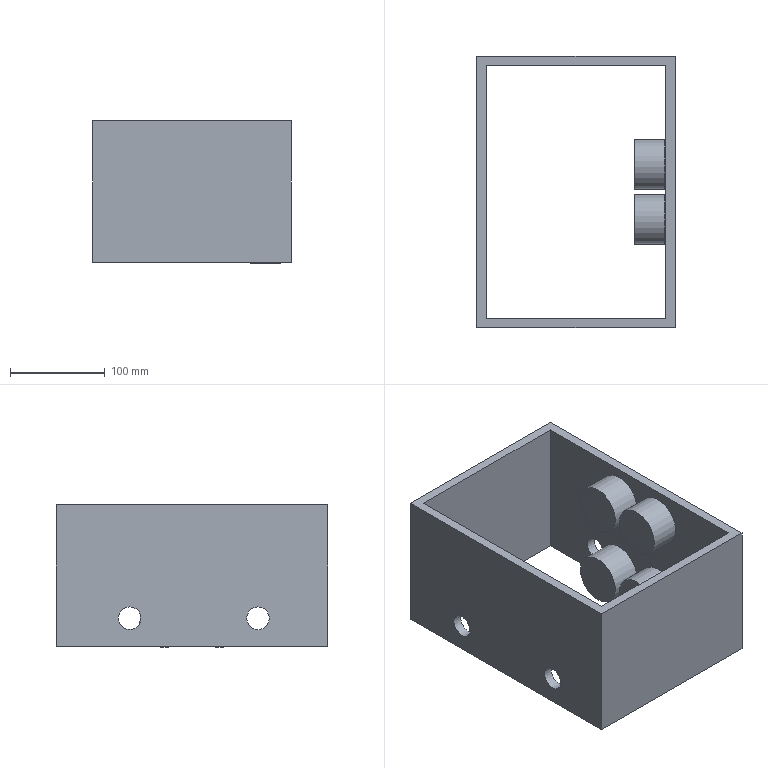Part | NX | features BREP 5 | 5 solids | 26 faces | box 209.8 x 286.897 x 151.129 mm | volume 1686526 mm3 | plane 18 | cylinder 8 | commonest cylinder face diameters 24 x4 52.257 x4
STEP:
#1=CARTESIAN_POINT('',(376.9,890.205,101.));
#2=VERTEX_POINT('',#1);
#3=CARTESIAN_POINT('',(376.9,864.077,101.));
#4=DIRECTION('',(1.,0.,0.));
#5=DIRECTION('',(0.,1.,0.));
#6=AXIS2_PLACEMENT_3D('',#3,#4,#5);
#7=CIRCLE('',#6,26.129);
#8=EDGE_CURVE('',#2,#2,#7,.T.);
#9=ORIENTED_EDGE('',*,*,#8,.T.);
#10=EDGE_LOOP('',(#9));
#11=FACE_BOUND('',#10,.T.);
#12=CARTESIAN_POINT('',(408.9,890.205,101.));
#13=VERTEX_POINT('',#12);
#14=CARTESIAN_POINT('',(408.9,864.077,101.));
#15=DIRECTION('',(1.,0.,0.));
#16=DIRECTION('',(0.,1.,0.));
#17=AXIS2_PLACEMENT_3D('',#14,#15,#16);
#18=CIRCLE('',#17,26.129);
#19=EDGE_CURVE('',#13,#13,#18,.T.);
#20=ORIENTED_EDGE('',*,*,#19,.F.);
#21=EDGE_LOOP('',(#20));
#22=FACE_BOUND('',#21,.T.);
#23=CARTESIAN_POINT('',(376.9,864.077,101.));
#24=DIRECTION('',(1.,0.,0.));
#25=DIRECTION('',(0.,0.,1.));
#26=AXIS2_PLACEMENT_3D('',#23,#24,#25);
#27=CYLINDRICAL_SURFACE('',#26,26.129);
#28=ADVANCED_FACE('',(#11,#22),#27,.T.);
#29=ORIENTED_EDGE('',*,*,#8,.F.);
#30=EDGE_LOOP('',(#29));
#31=FACE_BOUND('',#30,.T.);
#32=CARTESIAN_POINT('',(376.9,864.077,101.));
#33=DIRECTION('',(1.,0.,0.));
#34=DIRECTION('',(0.,0.,1.));
#35=AXIS2_PLACEMENT_3D('',#32,#33,#34);
#36=PLANE('',#35);
#37=ADVANCED_FACE('',(#31),#36,.F.);
#38=ORIENTED_EDGE('',*,*,#19,.T.);
#39=EDGE_LOOP('',(#38));
#40=FACE_BOUND('',#39,.T.);
#41=CARTESIAN_POINT('',(408.9,864.077,101.));
#42=DIRECTION('',(1.,0.,0.));
#43=DIRECTION('',(0.,0.,1.));
#44=AXIS2_PLACEMENT_3D('',#41,#42,#43);
#45=PLANE('',#44);
#46=ADVANCED_FACE('',(#40),#45,.T.);
#47=CLOSED_SHELL('',(#28,#37,#46));
#48=MANIFOLD_SOLID_BREP('',#47);
#49=CARTESIAN_POINT('',(210.1,691.509,136.));
#50=VERTEX_POINT('',#49);
#51=CARTESIAN_POINT('',(210.1,978.406,136.));
#52=VERTEX_POINT('',#51);
#53=CARTESIAN_POINT('',(210.1,943.406,136.));
#54=DIRECTION('',(0.,1.,0.));
#55=VECTOR('',#54,1000.);
#56=LINE('',#53,#55);
#57=EDGE_CURVE('',#50,#52,#56,.T.);
#58=ORIENTED_EDGE('',*,*,#57,.T.);
#59=CARTESIAN_POINT('',(210.1,978.406,-14.));
#60=VERTEX_POINT('',#59);
#61=CARTESIAN_POINT('',(210.1,978.406,-14.));
#62=DIRECTION('',(0.,0.,-1.));
#63=VECTOR('',#62,1000.);
#64=LINE('',#61,#63);
#65=EDGE_CURVE('',#52,#60,#64,.T.);
#66=ORIENTED_EDGE('',*,*,#65,.T.);
#67=CARTESIAN_POINT('',(210.1,691.509,-14.));
#68=VERTEX_POINT('',#67);
#69=CARTESIAN_POINT('',(210.1,943.406,-14.));
#70=DIRECTION('',(0.,-1.,0.));
#71=VECTOR('',#70,1000.);
#72=LINE('',#69,#71);
#73=EDGE_CURVE('',#60,#68,#72,.T.);
#74=ORIENTED_EDGE('',*,*,#73,.T.);
#75=CARTESIAN_POINT('',(210.1,691.509,-14.));
#76=DIRECTION('',(0.,0.,1.));
#77=VECTOR('',#76,1000.);
#78=LINE('',#75,#77);
#79=EDGE_CURVE('',#68,#50,#78,.T.);
#80=ORIENTED_EDGE('',*,*,#79,.T.);
#81=EDGE_LOOP('',(#58,#66,#74,#80));
#82=FACE_BOUND('',#81,.T.);
#83=CARTESIAN_POINT('',(210.1,765.15,27.85));
#84=VERTEX_POINT('',#83);
#85=CARTESIAN_POINT('',(210.1,765.15,15.85));
#86=DIRECTION('',(-1.,0.,0.));
#87=DIRECTION('',(0.,0.,1.));
#88=AXIS2_PLACEMENT_3D('',#85,#86,#87);
#89=CIRCLE('',#88,12.);
#90=EDGE_CURVE('',#84,#84,#89,.T.);
#91=ORIENTED_EDGE('',*,*,#90,.F.);
#92=EDGE_LOOP('',(#91));
#93=FACE_BOUND('',#92,.T.);
#94=CARTESIAN_POINT('',(210.1,900.853,27.85));
#95=VERTEX_POINT('',#94);
#96=CARTESIAN_POINT('',(210.1,900.853,15.85));
#97=DIRECTION('',(1.,0.,0.));
#98=DIRECTION('',(0.,0.,1.));
#99=AXIS2_PLACEMENT_3D('',#96,#97,#98);
#100=CIRCLE('',#99,12.);
#101=EDGE_CURVE('',#95,#95,#100,.T.);
#102=ORIENTED_EDGE('',*,*,#101,.T.);
#103=EDGE_LOOP('',(#102));
#104=FACE_BOUND('',#103,.T.);
#105=CARTESIAN_POINT('',(210.1,943.406,-14.));
#106=DIRECTION('',(-1.,0.,0.));
#107=DIRECTION('',(0.,0.,-1.));
#108=AXIS2_PLACEMENT_3D('',#105,#106,#107);
#109=PLANE('',#108);
#110=ADVANCED_FACE('',(#82,#93,#104),#109,.T.);
#111=CARTESIAN_POINT('',(419.9,978.406,136.));
#112=VERTEX_POINT('',#111);
#113=CARTESIAN_POINT('',(419.9,691.509,136.));
#114=VERTEX_POINT('',#113);
#115=CARTESIAN_POINT('',(419.9,726.509,136.));
#116=DIRECTION('',(0.,-1.,0.));
#117=VECTOR('',#116,1000.);
#118=LINE('',#115,#117);
#119=EDGE_CURVE('',#112,#114,#118,.T.);
#120=ORIENTED_EDGE('',*,*,#119,.T.);
#121=CARTESIAN_POINT('',(419.9,691.509,-14.));
#122=VERTEX_POINT('',#121);
#123=CARTESIAN_POINT('',(419.9,691.509,-14.));
#124=DIRECTION('',(0.,0.,1.));
#125=VECTOR('',#124,1000.);
#126=LINE('',#123,#125);
#127=EDGE_CURVE('',#122,#114,#126,.T.);
#128=ORIENTED_EDGE('',*,*,#127,.F.);
#129=CARTESIAN_POINT('',(419.9,978.406,-14.));
#130=VERTEX_POINT('',#129);
#131=CARTESIAN_POINT('',(419.9,923.406,-14.));
#132=DIRECTION('',(0.,1.,0.));
#133=VECTOR('',#132,1000.);
#134=LINE('',#131,#133);
#135=EDGE_CURVE('',#122,#130,#134,.T.);
#136=ORIENTED_EDGE('',*,*,#135,.T.);
#137=CARTESIAN_POINT('',(419.9,978.406,-14.));
#138=DIRECTION('',(0.,0.,1.));
#139=VECTOR('',#138,1000.);
#140=LINE('',#137,#139);
#141=EDGE_CURVE('',#130,#112,#140,.T.);
#142=ORIENTED_EDGE('',*,*,#141,.T.);
#143=EDGE_LOOP('',(#120,#128,#136,#142));
#144=FACE_BOUND('',#143,.T.);
#145=CARTESIAN_POINT('',(419.9,765.15,3.85));
#146=VERTEX_POINT('',#145);
#147=CARTESIAN_POINT('',(419.9,765.15,15.85));
#148=DIRECTION('',(1.,0.,0.));
#149=DIRECTION('',(0.,0.,-1.));
#150=AXIS2_PLACEMENT_3D('',#147,#148,#149);
#151=CIRCLE('',#150,12.);
#152=EDGE_CURVE('',#146,#146,#151,.T.);
#153=ORIENTED_EDGE('',*,*,#152,.F.);
#154=EDGE_LOOP('',(#153));
#155=FACE_BOUND('',#154,.T.);
#156=CARTESIAN_POINT('',(419.9,900.853,3.85));
#157=VERTEX_POINT('',#156);
#158=CARTESIAN_POINT('',(419.9,900.853,15.85));
#159=DIRECTION('',(-1.,0.,0.));
#160=DIRECTION('',(0.,0.,-1.));
#161=AXIS2_PLACEMENT_3D('',#158,#159,#160);
#162=CIRCLE('',#161,12.);
#163=EDGE_CURVE('',#157,#157,#162,.T.);
#164=ORIENTED_EDGE('',*,*,#163,.T.);
#165=EDGE_LOOP('',(#164));
#166=FACE_BOUND('',#165,.T.);
#167=CARTESIAN_POINT('',(419.9,726.509,-14.));
#168=DIRECTION('',(1.,0.,0.));
#169=DIRECTION('',(0.,0.,1.));
#170=AXIS2_PLACEMENT_3D('',#167,#168,#169);
#171=PLANE('',#170);
#172=ADVANCED_FACE('',(#144,#155,#166),#171,.T.);
#173=CARTESIAN_POINT('',(220.1,765.15,27.85));
#174=VERTEX_POINT('',#173);
#175=CARTESIAN_POINT('',(220.1,765.15,15.85));
#176=DIRECTION('',(-1.,0.,0.));
#177=DIRECTION('',(0.,0.,1.));
#178=AXIS2_PLACEMENT_3D('',#175,#176,#177);
#179=CIRCLE('',#178,12.);
#180=EDGE_CURVE('',#174,#174,#179,.T.);
#181=ORIENTED_EDGE('',*,*,#180,.T.);
#182=EDGE_LOOP('',(#181));
#183=FACE_BOUND('',#182,.T.);
#184=CARTESIAN_POINT('',(220.1,701.509,136.));
#185=VERTEX_POINT('',#184);
#186=CARTESIAN_POINT('',(220.1,968.406,136.));
#187=VERTEX_POINT('',#186);
#188=CARTESIAN_POINT('',(220.1,943.406,136.));
#189=DIRECTION('',(0.,1.,0.));
#190=VECTOR('',#189,1000.);
#191=LINE('',#188,#190);
#192=EDGE_CURVE('',#185,#187,#191,.T.);
#193=ORIENTED_EDGE('',*,*,#192,.F.);
#194=CARTESIAN_POINT('',(220.1,701.509,-14.));
#195=VERTEX_POINT('',#194);
#196=CARTESIAN_POINT('',(220.1,701.509,-14.));
#197=DIRECTION('',(0.,0.,1.));
#198=VECTOR('',#197,1000.);
#199=LINE('',#196,#198);
#200=EDGE_CURVE('',#195,#185,#199,.T.);
#201=ORIENTED_EDGE('',*,*,#200,.F.);
#202=CARTESIAN_POINT('',(220.1,968.406,-14.));
#203=VERTEX_POINT('',#202);
#204=CARTESIAN_POINT('',(220.1,943.406,-14.));
#205=DIRECTION('',(0.,-1.,0.));
#206=VECTOR('',#205,1000.);
#207=LINE('',#204,#206);
#208=EDGE_CURVE('',#203,#195,#207,.T.);
#209=ORIENTED_EDGE('',*,*,#208,.F.);
#210=CARTESIAN_POINT('',(220.1,968.406,-14.));
#211=DIRECTION('',(0.,0.,-1.));
#212=VECTOR('',#211,1000.);
#213=LINE('',#210,#212);
#214=EDGE_CURVE('',#187,#203,#213,.T.);
#215=ORIENTED_EDGE('',*,*,#214,.F.);
#216=EDGE_LOOP('',(#193,#201,#209,#215));
#217=FACE_BOUND('',#216,.T.);
#218=CARTESIAN_POINT('',(220.1,900.853,27.85));
#219=VERTEX_POINT('',#218);
#220=CARTESIAN_POINT('',(220.1,900.853,15.85));
#221=DIRECTION('',(1.,0.,0.));
#222=DIRECTION('',(0.,0.,1.));
#223=AXIS2_PLACEMENT_3D('',#220,#221,#222);
#224=CIRCLE('',#223,12.);
#225=EDGE_CURVE('',#219,#219,#224,.T.);
#226=ORIENTED_EDGE('',*,*,#225,.F.);
#227=EDGE_LOOP('',(#226));
#228=FACE_BOUND('',#227,.T.);
#229=CARTESIAN_POINT('',(220.1,943.406,-14.));
#230=DIRECTION('',(-1.,0.,0.));
#231=DIRECTION('',(0.,0.,-1.));
#232=AXIS2_PLACEMENT_3D('',#229,#230,#231);
#233=PLANE('',#232);
#234=ADVANCED_FACE('',(#183,#217,#228),#233,.F.);
#235=CARTESIAN_POINT('',(409.9,765.15,3.85));
#236=VERTEX_POINT('',#235);
#237=CARTESIAN_POINT('',(409.9,765.15,15.85));
#238=DIRECTION('',(1.,0.,0.));
#239=DIRECTION('',(0.,0.,-1.));
#240=AXIS2_PLACEMENT_3D('',#237,#238,#239);
#241=CIRCLE('',#240,12.);
#242=EDGE_CURVE('',#236,#236,#241,.T.);
#243=ORIENTED_EDGE('',*,*,#242,.T.);
#244=EDGE_LOOP('',(#243));
#245=FACE_BOUND('',#244,.T.);
#246=CARTESIAN_POINT('',(409.9,968.406,136.));
#247=VERTEX_POINT('',#246);
#248=CARTESIAN_POINT('',(409.9,701.509,136.));
#249=VERTEX_POINT('',#248);
#250=CARTESIAN_POINT('',(409.9,726.509,136.));
#251=DIRECTION('',(0.,-1.,0.));
#252=VECTOR('',#251,1000.);
#253=LINE('',#250,#252);
#254=EDGE_CURVE('',#247,#249,#253,.T.);
#255=ORIENTED_EDGE('',*,*,#254,.F.);
#256=CARTESIAN_POINT('',(409.9,968.406,-14.));
#257=VERTEX_POINT('',#256);
#258=CARTESIAN_POINT('',(409.9,968.406,-14.));
#259=DIRECTION('',(0.,0.,1.));
#260=VECTOR('',#259,1000.);
#261=LINE('',#258,#260);
#262=EDGE_CURVE('',#257,#247,#261,.T.);
#263=ORIENTED_EDGE('',*,*,#262,.F.);
#264=CARTESIAN_POINT('',(409.9,701.509,-14.));
#265=VERTEX_POINT('',#264);
#266=CARTESIAN_POINT('',(409.9,726.509,-14.));
#267=DIRECTION('',(0.,1.,0.));
#268=VECTOR('',#267,1000.);
#269=LINE('',#266,#268);
#270=EDGE_CURVE('',#265,#257,#269,.T.);
#271=ORIENTED_EDGE('',*,*,#270,.F.);
#272=CARTESIAN_POINT('',(409.9,701.509,-14.));
#273=DIRECTION('',(0.,0.,1.));
#274=VECTOR('',#273,1000.);
#275=LINE('',#272,#274);
#276=EDGE_CURVE('',#265,#249,#275,.T.);
#277=ORIENTED_EDGE('',*,*,#276,.T.);
#278=EDGE_LOOP('',(#255,#263,#271,#277));
#279=FACE_BOUND('',#278,.T.);
#280=CARTESIAN_POINT('',(409.9,900.853,3.85));
#281=VERTEX_POINT('',#280);
#282=CARTESIAN_POINT('',(409.9,900.853,15.85));
#283=DIRECTION('',(-1.,0.,0.));
#284=DIRECTION('',(0.,0.,-1.));
#285=AXIS2_PLACEMENT_3D('',#282,#283,#284);
#286=CIRCLE('',#285,12.);
#287=EDGE_CURVE('',#281,#281,#286,.T.);
#288=ORIENTED_EDGE('',*,*,#287,.F.);
#289=EDGE_LOOP('',(#288));
#290=FACE_BOUND('',#289,.T.);
#291=CARTESIAN_POINT('',(409.9,726.509,-14.));
#292=DIRECTION('',(1.,0.,0.));
#293=DIRECTION('',(0.,0.,1.));
#294=AXIS2_PLACEMENT_3D('',#291,#292,#293);
#295=PLANE('',#294);
#296=ADVANCED_FACE('',(#245,#279,#290),#295,.F.);
#297=CARTESIAN_POINT('',(419.9,978.406,136.));
#298=DIRECTION('',(1.,0.,0.));
#299=VECTOR('',#298,1000.);
#300=LINE('',#297,#299);
#301=EDGE_CURVE('',#52,#112,#300,.T.);
#302=ORIENTED_EDGE('',*,*,#301,.F.);
#303=ORIENTED_EDGE('',*,*,#57,.F.);
#304=CARTESIAN_POINT('',(210.1,691.509,136.));
#305=DIRECTION('',(-1.,0.,0.));
#306=VECTOR('',#305,1000.);
#307=LINE('',#304,#306);
#308=EDGE_CURVE('',#114,#50,#307,.T.);
#309=ORIENTED_EDGE('',*,*,#308,.F.);
#310=ORIENTED_EDGE('',*,*,#119,.F.);
#311=EDGE_LOOP('',(#302,#303,#309,#310));
#312=FACE_BOUND('',#311,.T.);
#313=ORIENTED_EDGE('',*,*,#192,.T.);
#314=CARTESIAN_POINT('',(419.9,968.406,136.));
#315=DIRECTION('',(1.,0.,0.));
#316=VECTOR('',#315,1000.);
#317=LINE('',#314,#316);
#318=EDGE_CURVE('',#187,#247,#317,.T.);
#319=ORIENTED_EDGE('',*,*,#318,.T.);
#320=ORIENTED_EDGE('',*,*,#254,.T.);
#321=CARTESIAN_POINT('',(210.1,701.509,136.));
#322=DIRECTION('',(-1.,0.,0.));
#323=VECTOR('',#322,1000.);
#324=LINE('',#321,#323);
#325=EDGE_CURVE('',#249,#185,#324,.T.);
#326=ORIENTED_EDGE('',*,*,#325,.T.);
#327=EDGE_LOOP('',(#313,#319,#320,#326));
#328=FACE_BOUND('',#327,.T.);
#329=CARTESIAN_POINT('',(210.1,943.406,136.));
#330=DIRECTION('',(0.,0.,-1.));
#331=DIRECTION('',(0.,1.,0.));
#332=AXIS2_PLACEMENT_3D('',#329,#330,#331);
#333=PLANE('',#332);
#334=ADVANCED_FACE('',(#312,#328),#333,.F.);
#335=CARTESIAN_POINT('',(419.9,978.406,-14.));
#336=DIRECTION('',(-1.,0.,0.));
#337=VECTOR('',#336,1000.);
#338=LINE('',#335,#337);
#339=EDGE_CURVE('',#130,#60,#338,.T.);
#340=ORIENTED_EDGE('',*,*,#339,.F.);
#341=ORIENTED_EDGE('',*,*,#135,.F.);
#342=CARTESIAN_POINT('',(210.1,691.509,-14.));
#343=DIRECTION('',(1.,0.,0.));
#344=VECTOR('',#343,1000.);
#345=LINE('',#342,#344);
#346=EDGE_CURVE('',#68,#122,#345,.T.);
#347=ORIENTED_EDGE('',*,*,#346,.F.);
#348=ORIENTED_EDGE('',*,*,#73,.F.);
#349=EDGE_LOOP('',(#340,#341,#347,#348));
#350=FACE_BOUND('',#349,.T.);
#351=ORIENTED_EDGE('',*,*,#270,.T.);
#352=CARTESIAN_POINT('',(419.9,968.406,-14.));
#353=DIRECTION('',(-1.,0.,0.));
#354=VECTOR('',#353,1000.);
#355=LINE('',#352,#354);
#356=EDGE_CURVE('',#257,#203,#355,.T.);
#357=ORIENTED_EDGE('',*,*,#356,.T.);
#358=ORIENTED_EDGE('',*,*,#208,.T.);
#359=CARTESIAN_POINT('',(210.1,701.509,-14.));
#360=DIRECTION('',(1.,0.,0.));
#361=VECTOR('',#360,1000.);
#362=LINE('',#359,#361);
#363=EDGE_CURVE('',#195,#265,#362,.T.);
#364=ORIENTED_EDGE('',*,*,#363,.T.);
#365=EDGE_LOOP('',(#351,#357,#358,#364));
#366=FACE_BOUND('',#365,.T.);
#367=CARTESIAN_POINT('',(419.9,923.406,-14.));
#368=DIRECTION('',(0.,0.,-1.));
#369=DIRECTION('',(0.,-1.,0.));
#370=AXIS2_PLACEMENT_3D('',#367,#368,#369);
#371=PLANE('',#370);
#372=ADVANCED_FACE('',(#350,#366),#371,.T.);
#373=ORIENTED_EDGE('',*,*,#301,.T.);
#374=ORIENTED_EDGE('',*,*,#141,.F.);
#375=ORIENTED_EDGE('',*,*,#339,.T.);
#376=ORIENTED_EDGE('',*,*,#65,.F.);
#377=EDGE_LOOP('',(#373,#374,#375,#376));
#378=FACE_BOUND('',#377,.T.);
#379=CARTESIAN_POINT('',(419.9,978.406,-14.));
#380=DIRECTION('',(0.,1.,0.));
#381=DIRECTION('',(0.,0.,-1.));
#382=AXIS2_PLACEMENT_3D('',#379,#380,#381);
#383=PLANE('',#382);
#384=ADVANCED_FACE('',(#378),#383,.T.);
#385=ORIENTED_EDGE('',*,*,#308,.T.);
#386=ORIENTED_EDGE('',*,*,#79,.F.);
#387=ORIENTED_EDGE('',*,*,#346,.T.);
#388=ORIENTED_EDGE('',*,*,#127,.T.);
#389=EDGE_LOOP('',(#385,#386,#387,#388));
#390=FACE_BOUND('',#389,.T.);
#391=CARTESIAN_POINT('',(210.1,691.509,-14.));
#392=DIRECTION('',(0.,-1.,0.));
#393=DIRECTION('',(0.,0.,1.));
#394=AXIS2_PLACEMENT_3D('',#391,#392,#393);
#395=PLANE('',#394);
#396=ADVANCED_FACE('',(#390),#395,.T.);
#397=ORIENTED_EDGE('',*,*,#318,.F.);
#398=ORIENTED_EDGE('',*,*,#214,.T.);
#399=ORIENTED_EDGE('',*,*,#356,.F.);
#400=ORIENTED_EDGE('',*,*,#262,.T.);
#401=EDGE_LOOP('',(#397,#398,#399,#400));
#402=FACE_BOUND('',#401,.T.);
#403=CARTESIAN_POINT('',(419.9,968.406,-14.));
#404=DIRECTION('',(0.,1.,0.));
#405=DIRECTION('',(0.,0.,-1.));
#406=AXIS2_PLACEMENT_3D('',#403,#404,#405);
#407=PLANE('',#406);
#408=ADVANCED_FACE('',(#402),#407,.F.);
#409=ORIENTED_EDGE('',*,*,#325,.F.);
#410=ORIENTED_EDGE('',*,*,#276,.F.);
#411=ORIENTED_EDGE('',*,*,#363,.F.);
#412=ORIENTED_EDGE('',*,*,#200,.T.);
#413=EDGE_LOOP('',(#409,#410,#411,#412));
#414=FACE_BOUND('',#413,.T.);
#415=CARTESIAN_POINT('',(210.1,701.509,-14.));
#416=DIRECTION('',(0.,-1.,0.));
#417=DIRECTION('',(0.,0.,1.));
#418=AXIS2_PLACEMENT_3D('',#415,#416,#417);
#419=PLANE('',#418);
#420=ADVANCED_FACE('',(#414),#419,.F.);
#421=ORIENTED_EDGE('',*,*,#152,.T.);
#422=EDGE_LOOP('',(#421));
#423=FACE_BOUND('',#422,.T.);
#424=ORIENTED_EDGE('',*,*,#242,.F.);
#425=EDGE_LOOP('',(#424));
#426=FACE_BOUND('',#425,.T.);
#427=CARTESIAN_POINT('',(465.1,765.15,15.85));
#428=DIRECTION('',(-1.,0.,0.));
#429=DIRECTION('',(0.,0.,-1.));
#430=AXIS2_PLACEMENT_3D('',#427,#428,#429);
#431=CYLINDRICAL_SURFACE('',#430,12.);
#432=ADVANCED_FACE('',(#423,#426),#431,.F.);
#433=ORIENTED_EDGE('',*,*,#163,.F.);
#434=EDGE_LOOP('',(#433));
#435=FACE_BOUND('',#434,.T.);
#436=ORIENTED_EDGE('',*,*,#287,.T.);
#437=EDGE_LOOP('',(#436));
#438=FACE_BOUND('',#437,.T.);
#439=CARTESIAN_POINT('',(465.1,900.853,15.85));
#440=DIRECTION('',(-1.,0.,0.));
#441=DIRECTION('',(0.,0.,-1.));
#442=AXIS2_PLACEMENT_3D('',#439,#440,#441);
#443=CYLINDRICAL_SURFACE('',#442,12.);
#444=ADVANCED_FACE('',(#435,#438),#443,.F.);
#445=ORIENTED_EDGE('',*,*,#90,.T.);
#446=EDGE_LOOP('',(#445));
#447=FACE_BOUND('',#446,.T.);
#448=ORIENTED_EDGE('',*,*,#180,.F.);
#449=EDGE_LOOP('',(#448));
#450=FACE_BOUND('',#449,.T.);
#451=CARTESIAN_POINT('',(465.1,765.15,15.85));
#452=DIRECTION('',(-1.,0.,0.));
#453=DIRECTION('',(0.,0.,-1.));
#454=AXIS2_PLACEMENT_3D('',#451,#452,#453);
#455=CYLINDRICAL_SURFACE('',#454,12.);
#456=ADVANCED_FACE('',(#447,#450),#455,.F.);
#457=ORIENTED_EDGE('',*,*,#101,.F.);
#458=EDGE_LOOP('',(#457));
#459=FACE_BOUND('',#458,.T.);
#460=ORIENTED_EDGE('',*,*,#225,.T.);
#461=EDGE_LOOP('',(#460));
#462=FACE_BOUND('',#461,.T.);
#463=CARTESIAN_POINT('',(465.1,900.853,15.85));
#464=DIRECTION('',(-1.,0.,0.));
#465=DIRECTION('',(0.,0.,-1.));
#466=AXIS2_PLACEMENT_3D('',#463,#464,#465);
#467=CYLINDRICAL_SURFACE('',#466,12.);
#468=ADVANCED_FACE('',(#459,#462),#467,.F.);
#469=CLOSED_SHELL('',(#110,#172,#234,#296,#334,#372,#384,#396,#408,#420,#432,#444,#456,#468));
#470=MANIFOLD_SOLID_BREP('',#469);
#471=CARTESIAN_POINT('',(376.9,831.967,11.));
#472=VERTEX_POINT('',#471);
#473=CARTESIAN_POINT('',(376.9,805.838,11.));
#474=DIRECTION('',(1.,0.,0.));
#475=DIRECTION('',(0.,1.,0.));
#476=AXIS2_PLACEMENT_3D('',#473,#474,#475);
#477=CIRCLE('',#476,26.129);
#478=EDGE_CURVE('',#472,#472,#477,.T.);
#479=ORIENTED_EDGE('',*,*,#478,.T.);
#480=EDGE_LOOP('',(#479));
#481=FACE_BOUND('',#480,.T.);
#482=CARTESIAN_POINT('',(408.9,831.967,11.));
#483=VERTEX_POINT('',#482);
#484=CARTESIAN_POINT('',(408.9,805.838,11.));
#485=DIRECTION('',(1.,0.,0.));
#486=DIRECTION('',(0.,1.,0.));
#487=AXIS2_PLACEMENT_3D('',#484,#485,#486);
#488=CIRCLE('',#487,26.129);
#489=EDGE_CURVE('',#483,#483,#488,.T.);
#490=ORIENTED_EDGE('',*,*,#489,.F.);
#491=EDGE_LOOP('',(#490));
#492=FACE_BOUND('',#491,.T.);
#493=CARTESIAN_POINT('',(376.9,805.838,11.));
#494=DIRECTION('',(1.,0.,0.));
#495=DIRECTION('',(0.,0.,1.));
#496=AXIS2_PLACEMENT_3D('',#493,#494,#495);
#497=CYLINDRICAL_SURFACE('',#496,26.129);
#498=ADVANCED_FACE('',(#481,#492),#497,.T.);
#499=ORIENTED_EDGE('',*,*,#478,.F.);
#500=EDGE_LOOP('',(#499));
#501=FACE_BOUND('',#500,.T.);
#502=CARTESIAN_POINT('',(376.9,805.838,11.));
#503=DIRECTION('',(1.,0.,0.));
#504=DIRECTION('',(0.,0.,1.));
#505=AXIS2_PLACEMENT_3D('',#502,#503,#504);
#506=PLANE('',#505);
#507=ADVANCED_FACE('',(#501),#506,.F.);
#508=ORIENTED_EDGE('',*,*,#489,.T.);
#509=EDGE_LOOP('',(#508));
#510=FACE_BOUND('',#509,.T.);
#511=CARTESIAN_POINT('',(408.9,805.838,11.));
#512=DIRECTION('',(1.,0.,0.));
#513=DIRECTION('',(0.,0.,1.));
#514=AXIS2_PLACEMENT_3D('',#511,#512,#513);
#515=PLANE('',#514);
#516=ADVANCED_FACE('',(#510),#515,.T.);
#517=CLOSED_SHELL('',(#498,#507,#516));
#518=MANIFOLD_SOLID_BREP('',#517);
#519=CARTESIAN_POINT('',(376.9,890.205,11.));
#520=VERTEX_POINT('',#519);
#521=CARTESIAN_POINT('',(376.9,864.077,11.));
#522=DIRECTION('',(1.,0.,0.));
#523=DIRECTION('',(0.,1.,0.));
#524=AXIS2_PLACEMENT_3D('',#521,#522,#523);
#525=CIRCLE('',#524,26.129);
#526=EDGE_CURVE('',#520,#520,#525,.T.);
#527=ORIENTED_EDGE('',*,*,#526,.T.);
#528=EDGE_LOOP('',(#527));
#529=FACE_BOUND('',#528,.T.);
#530=CARTESIAN_POINT('',(408.9,890.205,11.));
#531=VERTEX_POINT('',#530);
#532=CARTESIAN_POINT('',(408.9,864.077,11.));
#533=DIRECTION('',(1.,0.,0.));
#534=DIRECTION('',(0.,1.,0.));
#535=AXIS2_PLACEMENT_3D('',#532,#533,#534);
#536=CIRCLE('',#535,26.129);
#537=EDGE_CURVE('',#531,#531,#536,.T.);
#538=ORIENTED_EDGE('',*,*,#537,.F.);
#539=EDGE_LOOP('',(#538));
#540=FACE_BOUND('',#539,.T.);
#541=CARTESIAN_POINT('',(376.9,864.077,11.));
#542=DIRECTION('',(1.,0.,0.));
#543=DIRECTION('',(0.,0.,1.));
#544=AXIS2_PLACEMENT_3D('',#541,#542,#543);
#545=CYLINDRICAL_SURFACE('',#544,26.129);
#546=ADVANCED_FACE('',(#529,#540),#545,.T.);
#547=ORIENTED_EDGE('',*,*,#526,.F.);
#548=EDGE_LOOP('',(#547));
#549=FACE_BOUND('',#548,.T.);
#550=CARTESIAN_POINT('',(376.9,864.077,11.));
#551=DIRECTION('',(1.,0.,0.));
#552=DIRECTION('',(0.,0.,1.));
#553=AXIS2_PLACEMENT_3D('',#550,#551,#552);
#554=PLANE('',#553);
#555=ADVANCED_FACE('',(#549),#554,.F.);
#556=ORIENTED_EDGE('',*,*,#537,.T.);
#557=EDGE_LOOP('',(#556));
#558=FACE_BOUND('',#557,.T.);
#559=CARTESIAN_POINT('',(408.9,864.077,11.));
#560=DIRECTION('',(1.,0.,0.));
#561=DIRECTION('',(0.,0.,1.));
#562=AXIS2_PLACEMENT_3D('',#559,#560,#561);
#563=PLANE('',#562);
#564=ADVANCED_FACE('',(#558),#563,.T.);
#565=CLOSED_SHELL('',(#546,#555,#564));
#566=MANIFOLD_SOLID_BREP('',#565);
#567=CARTESIAN_POINT('',(376.9,831.967,101.));
#568=VERTEX_POINT('',#567);
#569=CARTESIAN_POINT('',(376.9,805.838,101.));
#570=DIRECTION('',(1.,0.,0.));
#571=DIRECTION('',(0.,1.,0.));
#572=AXIS2_PLACEMENT_3D('',#569,#570,#571);
#573=CIRCLE('',#572,26.129);
#574=EDGE_CURVE('',#568,#568,#573,.T.);
#575=ORIENTED_EDGE('',*,*,#574,.T.);
#576=EDGE_LOOP('',(#575));
#577=FACE_BOUND('',#576,.T.);
#578=CARTESIAN_POINT('',(408.9,831.967,101.));
#579=VERTEX_POINT('',#578);
#580=CARTESIAN_POINT('',(408.9,805.838,101.));
#581=DIRECTION('',(1.,0.,0.));
#582=DIRECTION('',(0.,1.,0.));
#583=AXIS2_PLACEMENT_3D('',#580,#581,#582);
#584=CIRCLE('',#583,26.129);
#585=EDGE_CURVE('',#579,#579,#584,.T.);
#586=ORIENTED_EDGE('',*,*,#585,.F.);
#587=EDGE_LOOP('',(#586));
#588=FACE_BOUND('',#587,.T.);
#589=CARTESIAN_POINT('',(376.9,805.838,101.));
#590=DIRECTION('',(1.,0.,0.));
#591=DIRECTION('',(0.,0.,1.));
#592=AXIS2_PLACEMENT_3D('',#589,#590,#591);
#593=CYLINDRICAL_SURFACE('',#592,26.129);
#594=ADVANCED_FACE('',(#577,#588),#593,.T.);
#595=ORIENTED_EDGE('',*,*,#574,.F.);
#596=EDGE_LOOP('',(#595));
#597=FACE_BOUND('',#596,.T.);
#598=CARTESIAN_POINT('',(376.9,805.838,101.));
#599=DIRECTION('',(1.,0.,0.));
#600=DIRECTION('',(0.,0.,1.));
#601=AXIS2_PLACEMENT_3D('',#598,#599,#600);
#602=PLANE('',#601);
#603=ADVANCED_FACE('',(#597),#602,.F.);
#604=ORIENTED_EDGE('',*,*,#585,.T.);
#605=EDGE_LOOP('',(#604));
#606=FACE_BOUND('',#605,.T.);
#607=CARTESIAN_POINT('',(408.9,805.838,101.));
#608=DIRECTION('',(1.,0.,0.));
#609=DIRECTION('',(0.,0.,1.));
#610=AXIS2_PLACEMENT_3D('',#607,#608,#609);
#611=PLANE('',#610);
#612=ADVANCED_FACE('',(#606),#611,.T.);
#613=CLOSED_SHELL('',(#594,#603,#612));
#614=MANIFOLD_SOLID_BREP('',#613);
#615=(LENGTH_UNIT()NAMED_UNIT(*)SI_UNIT(.MILLI.,.METRE.));
#616=UNCERTAINTY_MEASURE_WITH_UNIT(LENGTH_MEASURE(0.00001),#615,'','');
#617=(NAMED_UNIT(*)PLANE_ANGLE_UNIT()SI_UNIT($,.RADIAN.));
#618=(NAMED_UNIT(*)SI_UNIT($,.STERADIAN.)SOLID_ANGLE_UNIT());
#619=(GEOMETRIC_REPRESENTATION_CONTEXT(3)GLOBAL_UNCERTAINTY_ASSIGNED_CONTEXT((#616))GLOBAL_UNIT_ASSIGNED_CONTEXT((#615,#617,#618))REPRESENTATION_CONTEXT('',''));
#620=ADVANCED_BREP_SHAPE_REPRESENTATION('',(#48,#470,#518,#566,#614),#619);